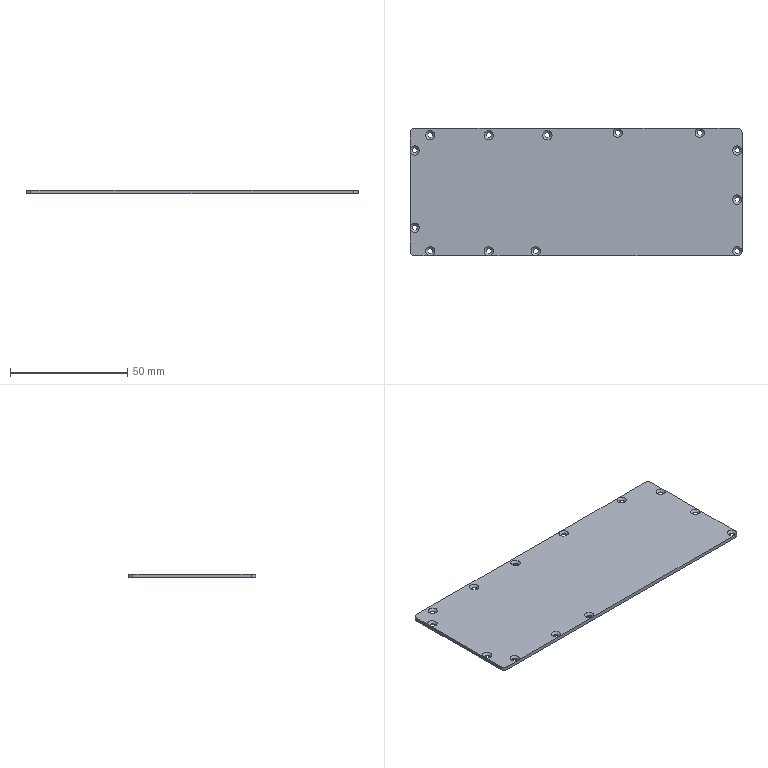Part | STEP file | Control module cover | 1 solid | 49 faces | box 141.709 x 54.52 x 1.5 mm | volume 11459 mm3 | cone 26 | cylinder 17 | plane 6 | commonest cylinder face diameters 2.2 x13 4 x4